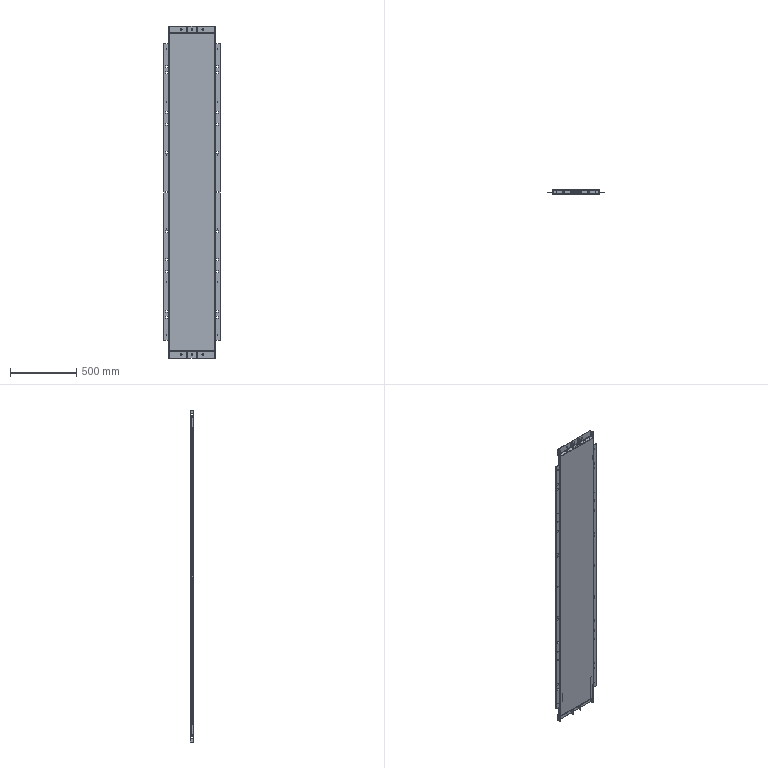Part | SolidWorks | 19 solids | 898 faces | box 428 x 30 x 2502 mm | volume 4227326 mm3 | plane 624 | cylinder 274 | commonest cylinder face diameters 5 x78 6.2 x44 6 x34 2 x24 4.2 x20 7 x16